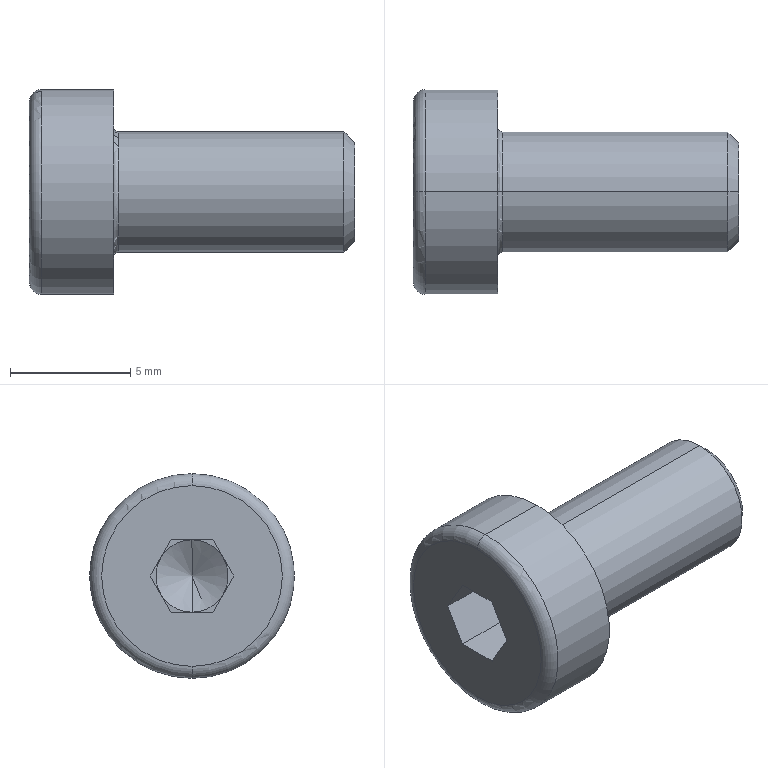Part | STEP file | socket head thin cap screw_din_DIN 7984 - M5 x 10 --- 7.6N | 1 solid | 27 faces | box 13.5 x 8.5 x 8.5 mm | volume 369.151 mm3 | plane 15 | cone 4 | torus 4 | cylinder 4 | commonest cylinder face diameters 5 x2 8.5 x2